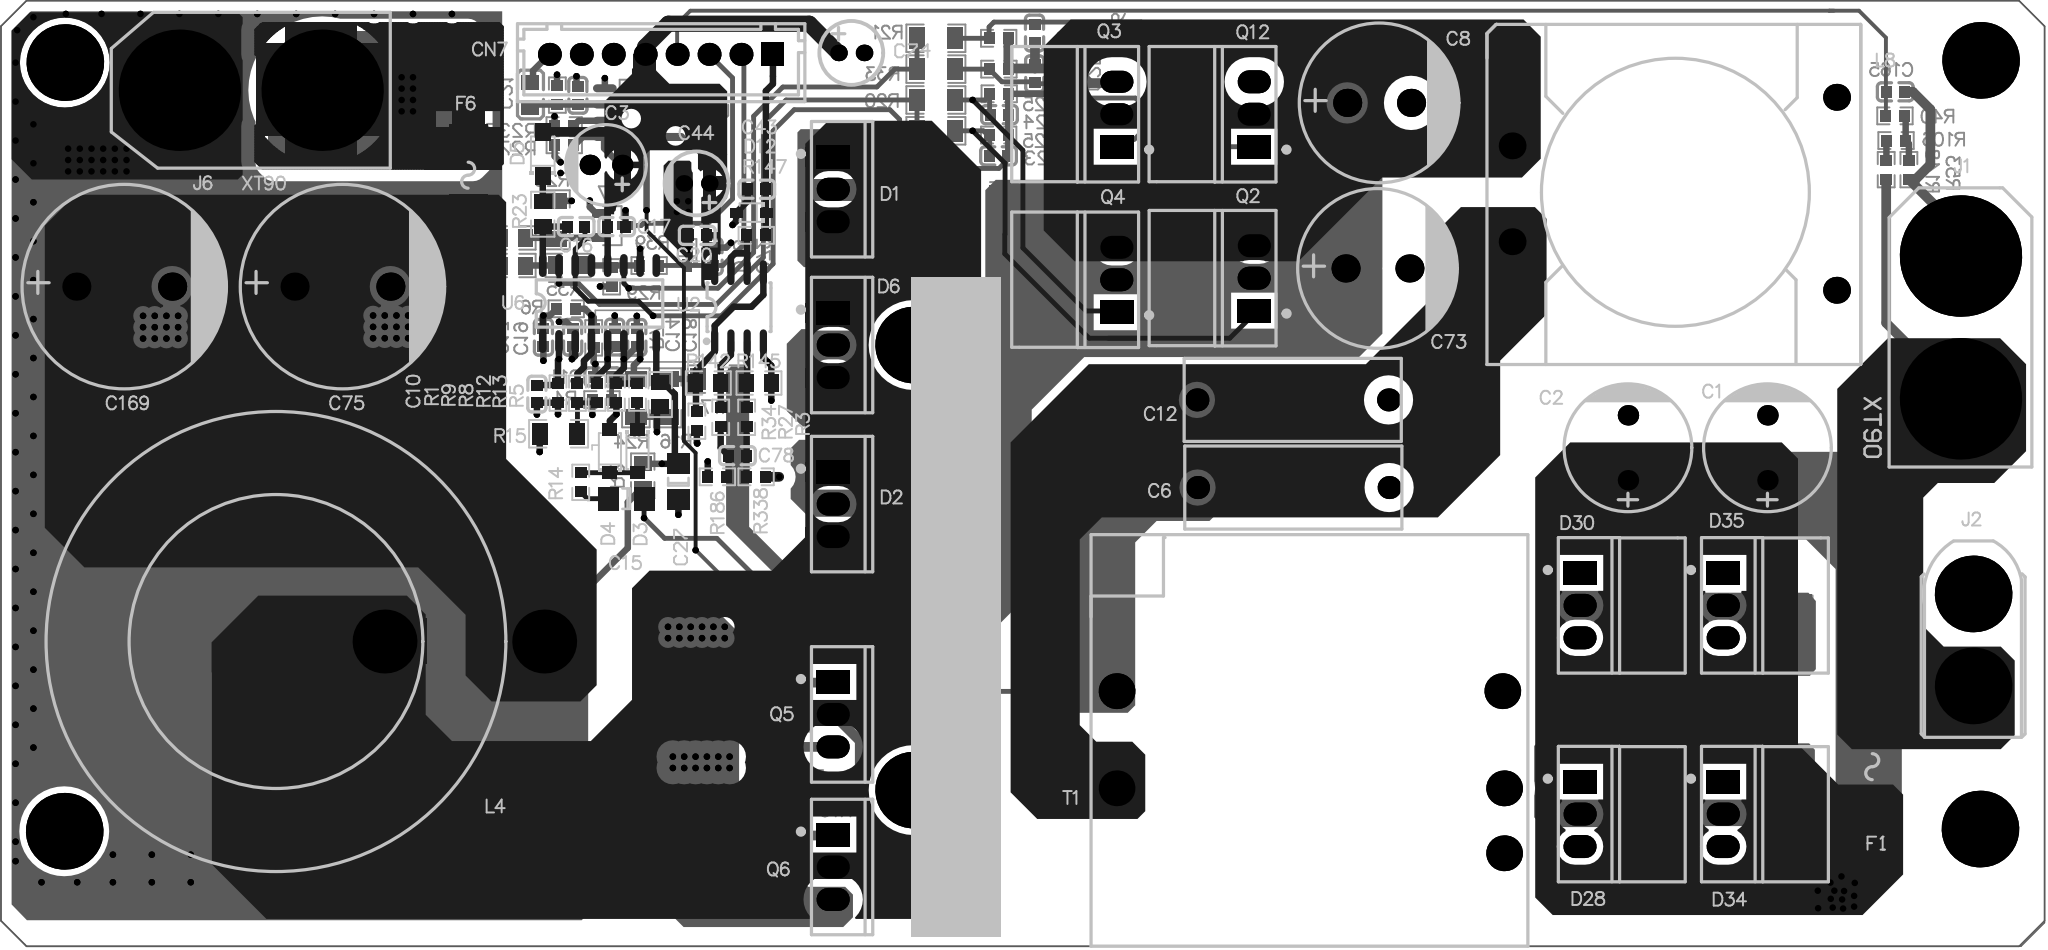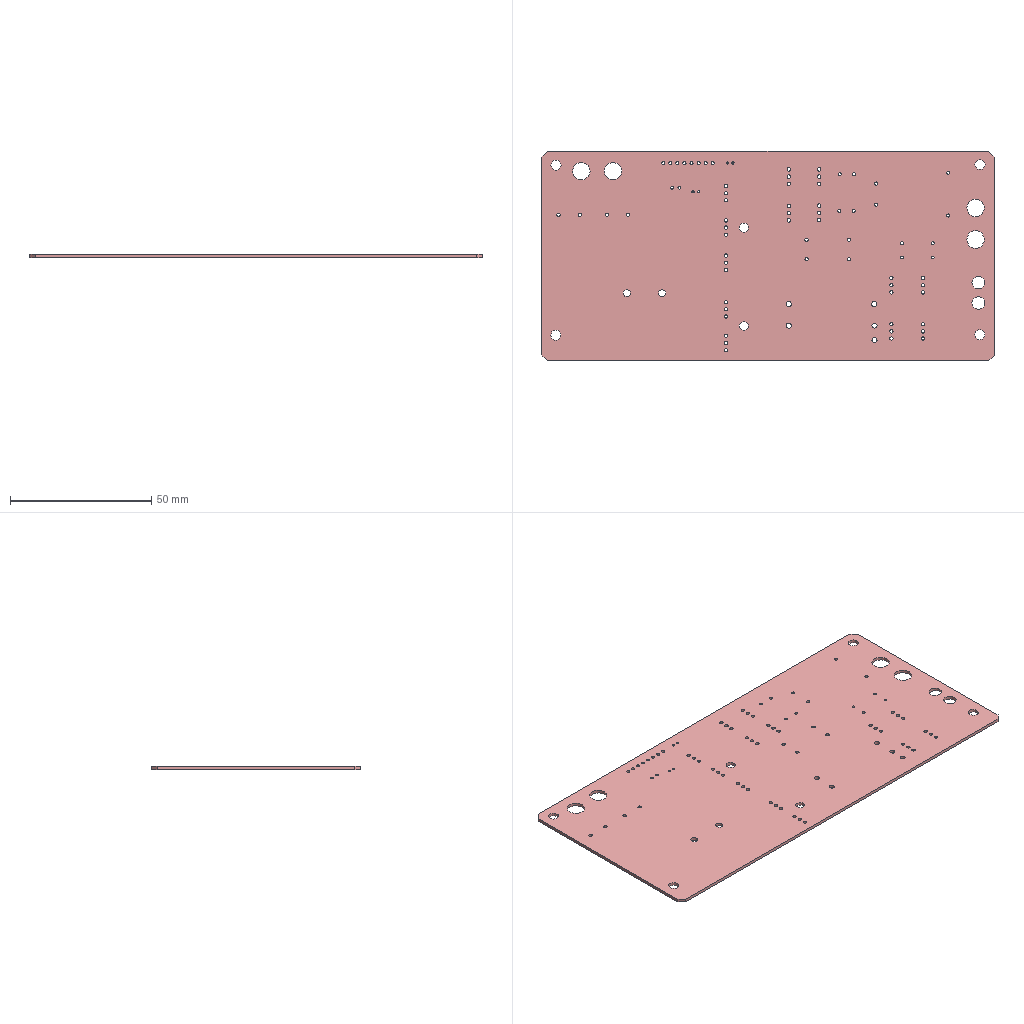Circuit board layout | Altium Designer | box 160 x 74 x 1.1 mm
Layer stack:
# Altium Designer layer stack of  (unit mm; dielectric type: 0 none, 1 core, 2 prepreg, 3 surface material)
index,name,kind,layer,copper_thickness_mm,dielectric_type,dielectric_thickness_mm,dielectric_material,dielectric_constant
0,Top Paste,other,,,,,,
1,Top Overlay,other,,,,,,
2,Top Solder,dielectric,,,3,0.0102,Solder Resist,3.5
3,Top Layer,copper,Top Layer,0.0356,,,,
4,Dielectric1,dielectric,,,1,0.32,FR-4,4.8
5,GND02,copper,GND02,0.0356,,,,
6,Dielectric2,dielectric,,,2,0.32,FR-4,4.8
7,PWR03,copper,PWR03,0.0356,,,,
8,Dielectric3,dielectric,,,1,0.32,FR-4,4.8
9,Bottom Layer,copper,Bottom Layer,0.0356,,,,
10,Bottom Solder,dielectric,,,3,0.0102,Solder Resist,3.5
11,Bottom Overlay,other,,,,,,
12,Bottom Paste,other,,,,,,
# drill layer pairs: low layer,high layer
drill_pair,Top Layer,Bottom Layer
Part placement:
Designator,Comment,Layer,Footprint,Center-X(mm),Center-Y(mm),Rotation
C169,560uF,TopLayer,CAP-TH_BD16.0-P7.50-D1.2-FD,-58.602,34.595,360
R2,,BottomLayer,R0805,-18.009,19.782,270
C27,10nF,TopLayer,C1206,-15.218,19.329,90
C12,150nF,TopLayer,CAP-TH_L17.0-W6.5-P15.00-D1.2,32.882,25.73,360
Q3,IRF640NPBF,TopLayer,TO-220-3_L10.0-W4.5-P2.54-L-N,19.11,48.082,90
Q12,IRF640NPBF,TopLayer,TO-220-3_L10.0-W4.5-P2.54-L-N,29.867,48.082,90
C8,150uF,TopLayer,CAP-TH_BD12.5-P5.00-D0.6-FD,39.646,48.971,360
Q2,IRF640NPBF,TopLayer,TO-220-3_L10.0-W4.5-P2.54-L-N,29.87,35.255,90
R34,1K,TopLayer,R0603,-13.771,24.063,270
Q6,KNP9120A,TopLayer,TO-220-3_L10.0-W4.5-P2.54-L,-3.094,-10.82,270
Q5,KNP9120A,TopLayer,TO-220-3_L10.0-W4.5-P2.54-L,-3.094,1.118,270
D6,SBD20C200T,TopLayer,TO-220-3_L10.0-W4.5-P2.54-L,-3.094,30.023,270
D2,SBD20C200T,TopLayer,TO-220-3_L10.0-W4.5-P2.54-L,-3.094,17.577,270
D1,SBD20C200T,TopLayer,TO-220-3_L10.0-W4.5-P2.54-L,-3.094,42.215,270
R14,,TopLayer,R0603,-22.864,19.279,90
R13,,TopLayer,R0603,-18.419,26.265,90
D4,1N4148W_C388533,TopLayer,SOD-123_L2.8-W1.8-LS3.7-RD,-20.578,21.725,90
D3,1N4148W_C388533,TopLayer,SOD-123_L2.8-W1.8-LS3.7-RD,-18.419,21.725,270
C15,NC,TopLayer,C1206,-19.305,18.001,180
D5,FR107_C2760867,TopLayer,SOD-123FL_L2.7-W1.8-LS3.8-RD,-25.835,44.966,90
R23,,TopLayer,R0805,-25.835,40.26,90
Q4,IRF640NPBF,TopLayer,TO-220-3_L10.0-W4.5-P2.54-L-N,19.11,35.128,90
D35,SBD20C200T,TopLayer,TO-220-3_L10.0-W4.5-P2.54-L-N,66.589,9.652,270
D34,SBD20C200T,TopLayer,TO-220-3_L10.0-W4.5-P2.54-L-N,66.589,-6.68,270
D30,SBD20C200T,TopLayer,TO-220-3_L10.0-W4.5-P2.54-L-N,55.38,9.652,270
D28,SBD20C200T,TopLayer,TO-220-3_L10.0-W4.5-P2.54-L-N,55.38,-6.68,270
C73,150uF,TopLayer,CAP-TH_BD12.5-P5.00-D0.6-FD,39.519,36.017,360
T1,,TopLayer,PQ3230_3:2:2-N,34.261,-3.404,270
L8,6.3uH,TopLayer,PQ2620-N,62.76,41.859,360
L4,230uH,TopLayer,IND-TH_CS343090*2-W231K,-31.973,6.824,360
U6,EG6599,TopLayer,SO-16_L10.0-W4.0-P1.27-LS6.2-BL,-21.39,33.274,360
R338,1,TopLayer,R0603,-9.134,19.711,360
R186,1,TopLayer,R0603,-12.165,19.711,180
R27,,TopLayer,R0603,-11.905,24.368,270
R12,,TopLayer,R0603,-20.07,26.265,90
R9,3.65K,TopLayer,R0603,-23.118,26.256,270
R8,,TopLayer,R0603,-21.586,26.263,90
R5,,TopLayer,R0805,-16.641,26.146,90
R3,,TopLayer,R0603,-9.873,24.368,270
R1,1.5M,TopLayer,R0603,-24.642,26.265,90
J6,10V-90V 400W 5.6A MAX,TopLayer,XT90,-48.696,49.962,360
J2,XT60,TopLayer,CONN-TH_XT60UPB-F,86.153,6.947,270
J1,,TopLayer,XT90N,85.162,31.4,270
F6,10A/200V,TopLayer,FUSE-SMD_L6.1-W2.5,-31.677,43.314,270
CN7,HX25003-8A,TopLayer,CONN-TH_8P-P2.50_HX25003-8A,-16.564,52.767,360
C78,100nF,TopLayer,C0603,-10.588,21.362,360
C75,560uF,TopLayer,CAP-TH_BD16.0-P7.50-D1.2-FD,-41.517,34.595,0
C10,220nF,TopLayer,C0603,-26.293,26.194,90
C3,220uF,TopLayer,CAP-TH_BD6.3-P2.50-D1.0-FD,-20.883,44.12,180
C2,390uF,TopLayer,CAP-TH_BD10.0-P5.00-D1.0-FD,59.127,21.984,90
C1,390uF,TopLayer,CAP-TH_BD10.0-P5.00-D1.0-FD,70.049,21.984,90
R15,10K,TopLayer,R1206,-24.596,23.081,180
C20,100nF,TopLayer,C0603,-13.748,38.608,180
C43,1nF,TopLayer,C0603,-9.072,42.215,360
C44,22uF,TopLayer,CAP-TH_BD5.0-P2.00-D0.8-FD,-13.794,42.672,180
D12,MM3Z3V3_C123917,TopLayer,SOD-323_L1.8-W1.3-LS2.5-RD,-9.522,40.386,180
R142,100K,TopLayer,R0805,-12.872,27.051,360
R145,100K,TopLayer,R0805,-8.907,27.051,360
R147,1K,TopLayer,R0603,-9.12,38.608,360
U2,EG358,TopLayer,SOIC-8_L5.0-W4.0-P1.27-LS6.0-BL,-10.469,32.982,360
C17,100nF,TopLayer,C0603,-20.056,39.294,180
C16,100nF,TopLayer,C0603,-23.231,39.294,180
R302,30K,BottomLayer,R0603,9.86,54.026,360
R33,10,BottomLayer,R1206,4.944,51.613,360
R32,30K,BottomLayer,R0603,9.878,51.613,360
R21,10,BottomLayer,R1206,4.944,54.026,360
R17,,BottomLayer,R1206,-12.165,27.356,180
R16,,BottomLayer,R1206,-16.056,25.892,270
R11,,BottomLayer,R1206,-52.333,27.356,360
C5,2.2nF,BottomLayer,C1206,-46.533,27.356,360
C6,150nF,TopLayer,CAP-TH_L17.0-W6.5-P15.00-D1.2,32.929,18.872,360
R148,560K,BottomLayer,R0603,79.346,43.748,270
R106,120K,BottomLayer,R0603,80.117,46.025,180
R53,30K,BottomLayer,R0603,81.124,43.748,90
R40,,BottomLayer,R0603,80.032,47.955,360
R39,,BottomLayer,R0603,-17.506,36.243,360
R35,0,BottomLayer,R0805,-23.853,36.249,180
R29,2K,BottomLayer,R0603,-20.443,35.364,270
R28,10K,BottomLayer,R1206,-24.799,39.823,90
R26,100K,BottomLayer,R0805,-28.155,36.246,180
R24,33K,BottomLayer,R1206,-18.546,25.892,90
R18,100K,BottomLayer,R0805,-28.155,38.405,180
R7,,BottomLayer,R0603,-21.848,30.582,270
R6,3K,BottomLayer,R0603,-23.998,32.86,180
R4,,BottomLayer,R0603,-21.201,25.75,360
Q7,MMBT3904,BottomLayer,SOT-23-3_L2.9-W1.3-P1.90-LS2.4-BR,-20.391,39.363,180
D15,MM3Z3V3_C123917,BottomLayer,SOD-323_L1.8-W1.3-LS2.5-RD,-14.533,37.421,90
C165,100nF,BottomLayer,C0603,80.046,49.835,180
C72,100nF,BottomLayer,C0603,-12.501,36.949,270
C19,1nF,BottomLayer,C0603,-23.499,30.639,90
C18,470pF,BottomLayer,C0603,-18.47,30.613,270
C14,2.2uF,BottomLayer,C0603,-20.197,30.636,270
C13,2.2uF,BottomLayer,C0603,-25.785,30.636,90
C11,1uF,BottomLayer,C0603,-21.148,27.526,180
R30,,BottomLayer,R2512,-14.126,2.279,270
R19,10,BottomLayer,R1206,4.944,46.787,360
R25,30K,BottomLayer,R0603,9.86,46.457,360
R47,,BottomLayer,R1206,2.912,12.497,360
R46,,BottomLayer,R2512,6.695,17.577,360
R45,,BottomLayer,R2512,6.676,40.818,360
R44,,BottomLayer,R2512,60.55,12.783,90
R43,,BottomLayer,R2512,71.624,12.936,90
R42,,BottomLayer,R2512,60.194,-9.804,270
R41,,BottomLayer,R2512,71.726,-9.594,270
R325,30K,BottomLayer,R0603,9.903,49.682,360
R22,,BottomLayer,R2512,6.517,23.597,360
R20,10,BottomLayer,R1206,4.944,49.2,360
C7,2.2nF,BottomLayer,C1206,8.331,12.497,360
R10,,BottomLayer,R1206,-2.927,-4.322,180
C4,2.2nF,BottomLayer,C1206,-7.065,-3,90
R98,30K,BottomLayer,R0603,-7.014,-10.947,90
R86,30K,BottomLayer,R0603,-6.836,0.8724,90
R73,10,BottomLayer,R1206,-7.358,3.772,360
R49,10,BottomLayer,R1206,-7.282,-8.039,360
C21,220pF,BottomLayer,C0603,-23.085,49.555,270
C74,22uF,TopLayer,CAP-TH_BD5.0-P2.00-D0.8-FD,-1.68,52.883,0
R237,,BottomLayer,R0603,-24.159,47.193,360
R271,,BottomLayer,R0603,-24.152,45.695,360
R295,NC,BottomLayer,R0603,-24.692,49.581,90
U18,EG3113,BottomLayer,SOP-8_L4.9-W3.9-P1.27-LS6.0-BL,-18.292,48.209,90
C9,2.2nF,BottomLayer,C0603,-8.712,-10.867,270
C22,2.2nF,BottomLayer,C0603,-8.563,0.9144,270
C23,2.2nF,BottomLayer,C0603,9.855,44.827,0
C24,2.2nF,BottomLayer,C0603,9.931,48.053,360
C25,2.2nF,BottomLayer,C0603,12.678,51.257,90
C26,2.2nF,BottomLayer,C0603,12.671,54.432,270
F1,20A/200V,TopLayer,FUSE-SMD_L6.1-W2.5,78.254,-2.972,90
L12,BLM21PG300SN1D,BottomLayer,L0805,-26.797,49.585,270
Pad and via stacks:
# Altium Designer via and pad stacks of  (unit mm). Each distinct definition once, with the count of objects using it.
# via: kind,start_layer,end_layer,hole_mm,diameter_mm,mode(0 simple;1 top-mid-bottom;2 full stack),diameter_per_layer,count,example_net
# pad: kind,layer,hole_mm,hole_type(0 round;1 square;2 slot),plating,top_size,top_shape(1 round;2 rect;3 octagon;9 rounded rect),mid_size,bottom_size,mode,footprint,size_per_layer,count,example
pad,Top Layer,0,0,plated,1.8x1.6,2,1.8x1.6,1.8x1.6,0,C1206,,4,C27.1
pad,Top Layer,0,0,plated,1.133x1.377,2,1.133x1.377,1.133x1.377,0,R0805,,8,R5.2
pad,Top Layer,0,0,plated,0.8065x0.864,2,0.8065x0.864,0.8065x0.864,0,R0603,,24,R34.2
pad,Top Layer,0,0,plated,0.95x1.15,2,0.95x1.15,0.95x1.15,0,SOD-123_L2.8-W1.8-LS3.7-RD,,4,D4.1
pad,Top Layer,0,0,plated,0.8x0.9,2,0.8x0.9,0.8x0.9,0,C0603,,12,C78.1
pad,Top Layer,0,0,plated,0.5684x1.95,1,0.5684x1.95,0.5684x1.95,0,SOIC-8_L5.0-W4.0-P1.27-LS6.0-BL,,8,U2.1
pad,Top Layer,0,0,plated,1x0.75,2,1x0.75,1x0.75,0,SOD-323_L1.8-W1.3-LS2.5-RD,,2,D12.1
pad,Top Layer,0,0,plated,1.208x1.701,2,1.208x1.701,1.208x1.701,0,R1206,,2,R15.2
pad,Top Layer,0,0,plated,2.5x3,2,2.5x3,2.5x3,0,FUSE-SMD_L6.1-W2.5,,4,F6.2
pad,Top Layer,0,0,plated,0.6x1.8,1,0.6x1.8,0.6x1.8,0,SO-16_L10.0-W4.0-P1.27-LS6.2-BL,,16,U6.1
pad,Top Layer,0,0,plated,1.4x1.2,2,1.4x1.2,1.4x1.2,0,SOD-123FL_L2.7-W1.8-LS3.8-RD,,2,D5.1
pad,Bottom Layer,0,0,plated,1.133x1.377,2,1.133x1.377,1.133x1.377,0,R0805,,8,R2.2
pad,Bottom Layer,0,0,plated,1.8x1.6,2,1.8x1.6,1.8x1.6,0,C1206,,6,C4.1
pad,Bottom Layer,0,0,plated,1.208x1.701,2,1.208x1.701,1.208x1.701,0,R1206,,26,R10.2
pad,Bottom Layer,0,0,plated,0.8065x0.864,2,0.8065x0.864,0.8065x0.864,0,R0603,,36,R86.2
pad,Bottom Layer,0,0,plated,1.282x3.456,2,1.282x3.456,1.282x3.456,0,R2512,,16,R44.2
pad,Bottom Layer,0,0,plated,0.8x0.9,2,0.8x0.9,0.8x0.9,0,C0603,,28,C165.1
pad,Bottom Layer,0,0,plated,1x0.75,2,1x0.75,1x0.75,0,SOD-323_L1.8-W1.3-LS2.5-RD,,2,D15.2
pad,Bottom Layer,0,0,plated,0.63x1.865,1,0.63x1.865,0.63x1.865,0,SOP-8_L4.9-W3.9-P1.27-LS6.0-BL,,8,U18.5
pad,Bottom Layer,0,0,plated,1.25x0.7,2,1.25x0.7,1.25x0.7,0,SOT-23-3_L2.9-W1.3-P1.90-LS2.4-BR,,3,Q7.1
pad,Bottom Layer,0,0,plated,1.133x1.377,2,1.133x1.377,1.133x1.377,0,L0805,,2,L12.1
pad,Multi-Layer,1.2,0,plated,2.2x2.2,1,2.2x2.2,2.2x2.2,0,CAP-TH_BD16.0-P7.50-D1.2-FD,,4,C169.2
pad,Multi-Layer,6.2,0,plated,9.5x9.5,1,9.5x9.5,9.5x9.5,0,XT90N,,2,J1.2
pad,Multi-Layer,4.5,0,plated,6x6,1,6x6,6x6,0,CONN-TH_XT60UPB-F,,2,J2.1
pad,Multi-Layer,1.8,0,plated,2.8x2.8,1,2.8x2.8,2.8x2.8,0,PQ3230 3:2:2-N,,5,T1.8
pad,Multi-Layer,1.2,0,plated,1.8x2.6,1,1.8x2.6,1.8x2.6,0,TO-220-3_L10.0-W4.5-P2.54-L-N,,14,Q12.2
pad,Multi-Layer,1.2,0,plated,1.8x2.6,2,1.8x2.6,1.8x2.6,0,TO-220-3_L10.0-W4.5-P2.54-L-N,,8,Q12.1
pad,Multi-Layer,1.2,0,plated,1.727x2.6,1,1.727x2.6,1.727x2.6,0,TO-220-3_L10.0-W4.5-P2.54-L-N,,2,Q3.2
pad,Multi-Layer,1.1,0,plated,2.2x2.2,1,2.2x2.2,2.2x2.2,0,CAP-TH_BD12.5-P5.00-D0.6-FD,,4,C8.2
pad,Multi-Layer,1.2,0,plated,1.8x2.6,2,1.8x2.6,1.8x2.6,0,TO-220-3_L10.0-W4.5-P2.54-L,,5,D6.1
pad,Multi-Layer,1.2,0,plated,1.8x2.6,1,1.8x2.6,1.8x2.6,0,TO-220-3_L10.0-W4.5-P2.54-L,,10,D6.3
pad,Multi-Layer,1,0,plated,1.6x1.6,1,1.6x1.6,1.6x1.6,0,CAP-TH_BD10.0-P5.00-D1.0-FD,,4,C2.1
pad,Multi-Layer,6.2,0,plated,9.5x9.5,1,9.5x9.5,9.5x9.5,0,XT90,,2,J6.1
pad,Multi-Layer,3.6,0,plated,6x6,1,6x6,6x6,0,,,4,0
pad,Multi-Layer,0.8,0,plated,1.3x1.3,1,1.3x1.3,1.3x1.3,0,CAP-TH_BD5.0-P2.00-D0.8-FD,,4,C44.1
pad,Multi-Layer,1.2,0,plated,1.8x1.8,1,1.8x1.8,1.8x1.8,0,CAP-TH_L17.0-W6.5-P15.00-D1.2,,4,C12.1
pad,Multi-Layer,3.2,0,plated,6x6,1,6x6,6x6,0,,,2,0
pad,Multi-Layer,1,0,plated,1.6x1.6,1,1.6x1.6,1.6x1.6,0,CAP-TH_BD6.3-P2.50-D1.0-FD,,2,C3.1
pad,Multi-Layer,1.1,0,plated,1.8x1.8,1,1.8x1.8,1.8x1.8,0,CONN-TH_8P-P2.50_HX25003-8A,,7,CN7.8
pad,Multi-Layer,1.1,0,plated,1.8x1.8,2,1.8x1.8,1.8x1.8,0,CONN-TH_8P-P2.50_HX25003-8A,,1,CN7.1
pad,Multi-Layer,2.5,0,plated,5x5,1,5x5,5x5,0,IND-TH_CS343090*2-W231K,,2,L4.1
pad,Multi-Layer,1.1,2,plated,2.1x2.1,1,2.1x2.1,2.1x2.1,0,PQ2620-N,,4,L8.3
via,Top Layer,Bottom Layer,0.254,0.508,0,,187,GND
via,Top Layer,Bottom Layer,0.3048,0.508,0,,13,NetC1_1
Copper pours:
name,layer,net,type(0 solid;1 hatched;2 none)
BottomLayer-No Net,Top Layer,NetC1_1,0
BottomLayer-No Net,Top Layer,B+,0
BottomLayer-No Net,Top Layer,PV-OVP,0
BottomLayer-No Net,Top Layer,NetD1_1,0
BottomLayer-No Net,Top Layer,NetL8_4,0
Bottom Layer-No Net 2,Top Layer,PV+,0
Bottom Layer-No Net 2,Top Layer,GND,0
Bottom Layer-No Net 2,Top Layer,+12V,0
BOTTOM-No Net,Top Layer,GND,0
Bottom Layer-No Net 2,Top Layer,+12V,0
BottomLayer-No Net,Top Layer,T1H,0
BottomLayer-No Net,GND02,BAT-,0
Bottom Layer-No Net 2,GND02,GND,0
BottomLayer-No Net,GND02,BAT-,0
BottomLayer-No Net,GND02,GND,0
BottomLayer-No Net,PWR03,NetD30_1,0
BottomLayer-No Net,PWR03,NetD28_1,0
Bottom Layer-No Net 2,PWR03,GND,0
BottomLayer-No Net,PWR03,BAT-,0
BottomLayer-No Net,PWR03,GND,0
BottomLayer-No Net,Bottom Layer,NetC1_1,0
BOTTOM-No Net,Bottom Layer,NetD30_2,0
BottomLayer-No Net,Bottom Layer,LLC_I,0
BOTTOM-No Net,Bottom Layer,NetD35_2,0
BOTTOM-No Net,Bottom Layer,NetD28_2,0
BOTTOM-No Net,Bottom Layer,NetD34_2,0
Bottom Layer-No Net 2,Bottom Layer,NetD1_2,0
Bottom Layer-No Net 2,Bottom Layer,PV+,0
Bottom Layer-No Net 2,Bottom Layer,GND,0
Bottom Layer-No Net 2,Bottom Layer,GND,0
BottomLayer-No Net,Bottom Layer,BAT-,0
BottomLayer-No Net,Bottom Layer,NetD6_2,0
BottomLayer-No Net,Bottom Layer,NetD2_2,0
BottomLayer-No Net,Bottom Layer,NetC7_2,0
Design rules, without the lines most boards share:
# Altium Designer design rules of  (exported by Altium Designer, unit mm)
# columns: name | kind | enabled | priority | scope1 | scope2 | descriptor | typed fields (field=value)
inpoly&inpoly | 0 | enabled | 2 | inpoly | inpoly | Clearance Constraint (Gap=20mil) (inpoly),(inpoly) | gap=0.508
inpoly&Net | 0 | enabled | 1 | inpoly | InNet('BAT-') or InNet('B+') or InNet('PV+')  or InNet('SW-PV') OR InNet('NETC75_1') | Clearance Constraint (Gap=40mil) (inpoly),(InNet('BAT-') or InNet('B+') or InNet('PV+')  or InNet('SW-PV') OR InNet('NETC75_1')) | gap=1.016
Clearance_2 | 0 | enabled | 4 | isvia | inpoly | Clearance Constraint (Gap=10mil) (isvia),(inpoly) | gap=0.254
INPOLY*All | 0 | enabled | 3 | INPOLY | All | Clearance Constraint (Gap=20mil) (INPOLY),(All) | gap=0.508
Clearance_1 | 0 | enabled | 5 | All | All | Clearance Constraint (Gap=8mil) (All),(All) | gap=0.2032
Width | 2 | enabled | 1 | All | All | Width Constraint (Min=10mil) (Max=500mil) (Preferred=10mil) (All) |
PlaneConnect | 6 | enabled | 1 | All | All | Power Plane Connect Rule(Relief Connect )(Expansion=8mil) (Conductor Width=10mil) (Air Gap=10mil) (Entries=4) (All) | relief_conductor_width=0.254 relief_entries=4 relief_expansion=0.2032
RoutingVias | 11 | enabled | 1 | All | All | Routing Via (MinHoleWidth=10mil) (MaxHoleWidth=10mil) (PreferredHoleWidth=10mil) (MinWidth=20mil) (MaxWidth=20mil) (PreferedWidth=20mil) (All) | via_min_hole=0.254 via_max_hole=0.254 via_preferred_diameter=0.508 via_preferred_hole=0.254
PlaneClearance | 12 | enabled | 1 | All | All | Power Plane Clearance (Clearance =12mil) (All) | clearance=0.3048
SolderMaskExpansion | 13 | enabled | 1 | All | All | Solder Mask Expansion (Expansion =2.5mil) (All) | expansion=0.0635
PolygonConnect_1 | 20 | enabled | 1 | ISVIA | All | Polygon Connect Rule(Direct Connect )(Conductor Width=10mil) (Relief Angle=90 Angle) (Entries=4) (Air Gap Width=10mil) (ISVIA),(All) | connect_style(0=relief,1=direct,2=none)=1 relief_conductor_width=0.254 relief_entries=4
PolygonConnect | 20 | enabled | 2 | All | All | Polygon Connect Rule(Direct Connect )(Conductor Width=20mil) (Relief Angle=90 Angle) (Entries=4) (Air Gap Width=10mil) (All),(All) | connect_style(0=relief,1=direct,2=none)=1 relief_conductor_width=0.508 relief_entries=4
ComponentClearance | 24 | disabled | 1 | All | All | Component Clearance Constraint ( Horizontal Gap = 10mil, Vertical Gap = 10mil ) (Disabled)(All),(All)  | gap=0.254
HoleSize | 42 | disabled | 1 | All | All | Hole Size Constraint (Min=1mil) (Max=100mil) (Disabled)(All) |
Testpoint | 43 | enabled | 1 | (IsPad And (OnTopLayer Or OnBottomLayer)) | All | Fabrication Testpoint Style (Under Component=Yes) ((IsPad And (OnTopLayer Or OnBottomLayer))) |
TestPointUsage | 44 | enabled | 1 | All | All | Fabrication Testpoint Usage (Valid =One Required, Allow multiple per net=No) (All) |
LayerPairs | 48 | disabled | 1 | All | All | Pads and Vias to follow the Drill pairs settings |
Height | 50 | disabled | 1 | All | All | Height Constraint (Min=0mil) (Max=1000mil) (Prefered=500mil) (Disabled)(All) | min_height=0 max_height=25.4
DiffPairsRouting | 51 | enabled | 1 | All | All | Differential Pairs Uncoupled Length using the Gap Constraints (Min=10mil) (Max=10mil) (Prefered=10mil)  and Width Constraints (Min=15mil) (Max=15mil) (Prefered=15mil) (All) |
HoleToHoleClearance | 52 | disabled | 1 | All | All | Hole To Hole Clearance (Gap=10mil) (Disabled)(All),(All) | gap=0.254
MinimumSolderMaskSliver | 53 | disabled | 1 | All | All | Minimum Solder Mask Sliver (Gap=10mil) (Disabled)(All),(All) |
SilkscreenOverComponentPads | 54 | disabled | 1 | IsPad | All | Silk To Solder Mask (Clearance=10mil) (Disabled)(IsPad),(All) |
SilkToSilkClearance | 55 | disabled | 1 | All | All | Silk to Silk (Clearance=10mil) (Disabled)(All),(All) |
NetAntennae | 56 | enabled | 1 | All | All | Net Antennae (Tolerance=1mil) (All) |
Classes set for this board:
# Altium Designer classes of  (member kind: 0 net, 1 component, 2 from-to, 3 pad, 4 layer, 5 differential pair, 6 design channel, 7 polygon, 8 structure, 9 xSignal)
# columns: class name | member kind | superclass | members
400W_2022-10-14 | 1 | no | C1; C2; C3; C4; C5; C6; C8; C10; C11; C12; C13; C14; C15; C16; C17; C18; C19; C20; C43; C44; C72; C73; C75; C78; C165; C169; CN7; D3; D4; D5; D12; D15; D28; D30; D34; D35; F6; J1; J2; J6; L4; L8; Q2; Q3; Q4; Q7; Q12; R1; R3; R4; R5; R6; R7; R8; R9; R10; R11; R12; R13; R14; R15; R16; R17; R18; R19; R20; R21; R22; R23; R24; R25; R26; R27; R28; R29; R30; R32; R33; R35; R39; R40; R49; R53; R73; R86; R98; R106; R142; R145; R147; R148; R186; R302; R325; R338; T1; U2; U6; U2; Q2; Q3; C7; D1; D2; D6; Q5; Q6; R34; R41; R42; R43; R44; R45; R46; R47; C12; R302; C21; C74; R237; R271; R295; U18; C9; C22; C23; C24; C25; C26; F1; L12; C27; R2;